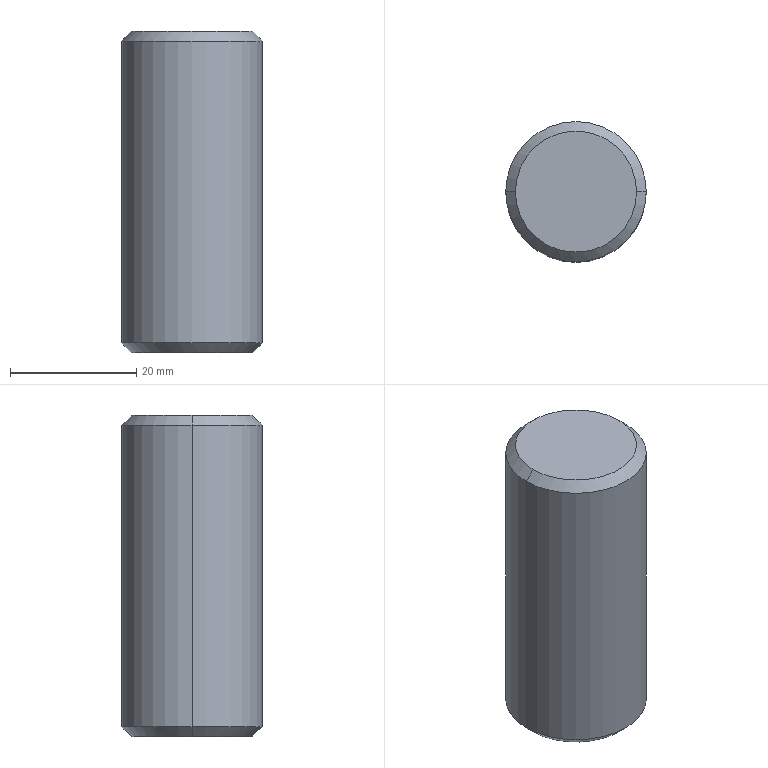Part | SolidWorks | features Chamfer 1, Extrusion 1 | 1 solid | 8 faces | box 22.225 x 22.225 x 50.8 mm | volume 19553 mm3 | cone 4 | cylinder 2 | plane 2 | commonest cylinder face diameters 22.225 x2
STEP:
#1=CARTESIAN_POINT('',(-9.588,0.,-25.4));
#2=VERTEX_POINT('',#1);
#3=CARTESIAN_POINT('',(9.588,0.,-25.4));
#4=VERTEX_POINT('',#3);
#5=CARTESIAN_POINT('',(0.,0.,-25.4));
#6=DIRECTION('',(0.,0.,-1.));
#7=DIRECTION('',(1.,0.,0.));
#8=AXIS2_PLACEMENT_3D('',#5,#6,#7);
#9=CIRCLE('',#8,9.588);
#10=EDGE_CURVE('',#2,#4,#9,.T.);
#11=ORIENTED_EDGE('',*,*,#10,.F.);
#12=CARTESIAN_POINT('',(-11.112,0.,-23.876));
#13=VERTEX_POINT('',#12);
#14=CARTESIAN_POINT('',(-11.112,0.,-23.876));
#15=DIRECTION('',(-0.7071,0.,0.7071));
#16=VECTOR('',#15,1000.);
#17=LINE('',#14,#16);
#18=EDGE_CURVE('',#2,#13,#17,.T.);
#19=ORIENTED_EDGE('',*,*,#18,.T.);
#20=CARTESIAN_POINT('',(11.112,0.,-23.876));
#21=VERTEX_POINT('',#20);
#22=CARTESIAN_POINT('',(0.,0.,-23.876));
#23=DIRECTION('',(0.,0.,1.));
#24=DIRECTION('',(1.,0.,0.));
#25=AXIS2_PLACEMENT_3D('',#22,#23,#24);
#26=CIRCLE('',#25,11.112);
#27=EDGE_CURVE('',#21,#13,#26,.T.);
#28=ORIENTED_EDGE('',*,*,#27,.F.);
#29=CARTESIAN_POINT('',(11.112,0.,-23.876));
#30=DIRECTION('',(0.7071,0.,0.7071));
#31=VECTOR('',#30,1000.);
#32=LINE('',#29,#31);
#33=EDGE_CURVE('',#4,#21,#32,.T.);
#34=ORIENTED_EDGE('',*,*,#33,.F.);
#35=EDGE_LOOP('',(#11,#19,#28,#34));
#36=FACE_OUTER_BOUND('',#35,.T.);
#37=CARTESIAN_POINT('',(0.,0.,-23.876));
#38=DIRECTION('',(0.,0.,1.));
#39=DIRECTION('',(1.,0.,0.));
#40=AXIS2_PLACEMENT_3D('',#37,#38,#39);
#41=CONICAL_SURFACE('',#40,11.112,0.7854);
#42=ADVANCED_FACE('',(#36),#41,.T.);
#43=CARTESIAN_POINT('',(9.588,0.,25.4));
#44=VERTEX_POINT('',#43);
#45=CARTESIAN_POINT('',(-9.588,0.,25.4));
#46=VERTEX_POINT('',#45);
#47=CARTESIAN_POINT('',(0.,0.,25.4));
#48=DIRECTION('',(0.,0.,1.));
#49=DIRECTION('',(1.,0.,0.));
#50=AXIS2_PLACEMENT_3D('',#47,#48,#49);
#51=CIRCLE('',#50,9.588);
#52=EDGE_CURVE('',#44,#46,#51,.T.);
#53=ORIENTED_EDGE('',*,*,#52,.F.);
#54=CARTESIAN_POINT('',(11.112,0.,23.876));
#55=VERTEX_POINT('',#54);
#56=CARTESIAN_POINT('',(9.588,0.,25.4));
#57=DIRECTION('',(0.7071,0.,-0.7071));
#58=VECTOR('',#57,1000.);
#59=LINE('',#56,#58);
#60=EDGE_CURVE('',#44,#55,#59,.T.);
#61=ORIENTED_EDGE('',*,*,#60,.T.);
#62=CARTESIAN_POINT('',(-11.112,0.,23.876));
#63=VERTEX_POINT('',#62);
#64=CARTESIAN_POINT('',(0.,0.,23.876));
#65=DIRECTION('',(0.,0.,-1.));
#66=DIRECTION('',(1.,0.,0.));
#67=AXIS2_PLACEMENT_3D('',#64,#65,#66);
#68=CIRCLE('',#67,11.112);
#69=EDGE_CURVE('',#63,#55,#68,.T.);
#70=ORIENTED_EDGE('',*,*,#69,.F.);
#71=CARTESIAN_POINT('',(-9.588,0.,25.4));
#72=DIRECTION('',(-0.7071,0.,-0.7071));
#73=VECTOR('',#72,1000.);
#74=LINE('',#71,#73);
#75=EDGE_CURVE('',#46,#63,#74,.T.);
#76=ORIENTED_EDGE('',*,*,#75,.F.);
#77=EDGE_LOOP('',(#53,#61,#70,#76));
#78=FACE_OUTER_BOUND('',#77,.T.);
#79=CARTESIAN_POINT('',(0.,0.,25.4));
#80=DIRECTION('',(0.,0.,-1.));
#81=DIRECTION('',(-1.,0.,0.));
#82=AXIS2_PLACEMENT_3D('',#79,#80,#81);
#83=CONICAL_SURFACE('',#82,9.588,0.7854);
#84=ADVANCED_FACE('',(#78),#83,.T.);
#85=ORIENTED_EDGE('',*,*,#69,.T.);
#86=CARTESIAN_POINT('',(11.112,0.,25.4));
#87=DIRECTION('',(0.,0.,-1.));
#88=VECTOR('',#87,1000.);
#89=LINE('',#86,#88);
#90=EDGE_CURVE('',#55,#21,#89,.T.);
#91=ORIENTED_EDGE('',*,*,#90,.T.);
#92=ORIENTED_EDGE('',*,*,#27,.T.);
#93=CARTESIAN_POINT('',(-11.112,0.,25.4));
#94=DIRECTION('',(0.,0.,-1.));
#95=VECTOR('',#94,1000.);
#96=LINE('',#93,#95);
#97=EDGE_CURVE('',#63,#13,#96,.T.);
#98=ORIENTED_EDGE('',*,*,#97,.F.);
#99=EDGE_LOOP('',(#85,#91,#92,#98));
#100=FACE_OUTER_BOUND('',#99,.T.);
#101=CARTESIAN_POINT('',(0.,0.,25.4));
#102=DIRECTION('',(0.,0.,-1.));
#103=DIRECTION('',(-1.,0.,0.));
#104=AXIS2_PLACEMENT_3D('',#101,#102,#103);
#105=CYLINDRICAL_SURFACE('',#104,11.112);
#106=ADVANCED_FACE('',(#100),#105,.T.);
#107=ORIENTED_EDGE('',*,*,#90,.F.);
#108=CARTESIAN_POINT('',(0.,0.,23.876));
#109=DIRECTION('',(0.,0.,-1.));
#110=DIRECTION('',(1.,0.,0.));
#111=AXIS2_PLACEMENT_3D('',#108,#109,#110);
#112=CIRCLE('',#111,11.112);
#113=EDGE_CURVE('',#55,#63,#112,.T.);
#114=ORIENTED_EDGE('',*,*,#113,.T.);
#115=ORIENTED_EDGE('',*,*,#97,.T.);
#116=CARTESIAN_POINT('',(0.,0.,-23.876));
#117=DIRECTION('',(0.,0.,1.));
#118=DIRECTION('',(1.,0.,0.));
#119=AXIS2_PLACEMENT_3D('',#116,#117,#118);
#120=CIRCLE('',#119,11.112);
#121=EDGE_CURVE('',#13,#21,#120,.T.);
#122=ORIENTED_EDGE('',*,*,#121,.T.);
#123=EDGE_LOOP('',(#107,#114,#115,#122));
#124=FACE_OUTER_BOUND('',#123,.T.);
#125=CARTESIAN_POINT('',(0.,0.,25.4));
#126=DIRECTION('',(0.,0.,-1.));
#127=DIRECTION('',(-1.,0.,0.));
#128=AXIS2_PLACEMENT_3D('',#125,#126,#127);
#129=CYLINDRICAL_SURFACE('',#128,11.112);
#130=ADVANCED_FACE('',(#124),#129,.T.);
#131=CARTESIAN_POINT('',(0.,0.,25.4));
#132=DIRECTION('',(0.,0.,1.));
#133=DIRECTION('',(1.,0.,0.));
#134=AXIS2_PLACEMENT_3D('',#131,#132,#133);
#135=CIRCLE('',#134,9.588);
#136=EDGE_CURVE('',#46,#44,#135,.T.);
#137=ORIENTED_EDGE('',*,*,#136,.T.);
#138=ORIENTED_EDGE('',*,*,#52,.T.);
#139=EDGE_LOOP('',(#137,#138));
#140=FACE_OUTER_BOUND('',#139,.T.);
#141=CARTESIAN_POINT('',(0.,0.,25.4));
#142=DIRECTION('',(0.,0.,1.));
#143=DIRECTION('',(1.,0.,0.));
#144=AXIS2_PLACEMENT_3D('',#141,#142,#143);
#145=PLANE('',#144);
#146=ADVANCED_FACE('',(#140),#145,.T.);
#147=CARTESIAN_POINT('',(0.,0.,-25.4));
#148=DIRECTION('',(0.,0.,-1.));
#149=DIRECTION('',(1.,0.,0.));
#150=AXIS2_PLACEMENT_3D('',#147,#148,#149);
#151=CIRCLE('',#150,9.588);
#152=EDGE_CURVE('',#4,#2,#151,.T.);
#153=ORIENTED_EDGE('',*,*,#152,.T.);
#154=ORIENTED_EDGE('',*,*,#10,.T.);
#155=EDGE_LOOP('',(#153,#154));
#156=FACE_OUTER_BOUND('',#155,.T.);
#157=CARTESIAN_POINT('',(0.,0.,-25.4));
#158=DIRECTION('',(0.,0.,1.));
#159=DIRECTION('',(1.,0.,0.));
#160=AXIS2_PLACEMENT_3D('',#157,#158,#159);
#161=PLANE('',#160);
#162=ADVANCED_FACE('',(#156),#161,.F.);
#163=ORIENTED_EDGE('',*,*,#60,.F.);
#164=ORIENTED_EDGE('',*,*,#136,.F.);
#165=ORIENTED_EDGE('',*,*,#75,.T.);
#166=ORIENTED_EDGE('',*,*,#113,.F.);
#167=EDGE_LOOP('',(#163,#164,#165,#166));
#168=FACE_OUTER_BOUND('',#167,.T.);
#169=CARTESIAN_POINT('',(0.,0.,25.4));
#170=DIRECTION('',(0.,0.,-1.));
#171=DIRECTION('',(-1.,0.,0.));
#172=AXIS2_PLACEMENT_3D('',#169,#170,#171);
#173=CONICAL_SURFACE('',#172,9.588,0.7854);
#174=ADVANCED_FACE('',(#168),#173,.T.);
#175=ORIENTED_EDGE('',*,*,#18,.F.);
#176=ORIENTED_EDGE('',*,*,#152,.F.);
#177=ORIENTED_EDGE('',*,*,#33,.T.);
#178=ORIENTED_EDGE('',*,*,#121,.F.);
#179=EDGE_LOOP('',(#175,#176,#177,#178));
#180=FACE_OUTER_BOUND('',#179,.T.);
#181=CARTESIAN_POINT('',(0.,0.,-23.876));
#182=DIRECTION('',(0.,0.,1.));
#183=DIRECTION('',(1.,0.,0.));
#184=AXIS2_PLACEMENT_3D('',#181,#182,#183);
#185=CONICAL_SURFACE('',#184,11.112,0.7854);
#186=ADVANCED_FACE('',(#180),#185,.T.);
#187=CLOSED_SHELL('',(#42,#84,#106,#130,#146,#162,#174,#186));
#188=MANIFOLD_SOLID_BREP('',#187);
#189=CARTESIAN_POINT('',(0.,0.,0.));
#190=DIRECTION('',(0.,0.,1.));
#191=DIRECTION('',(1.,0.,0.));
#192=AXIS2_PLACEMENT_3D('',#189,#190,#191);
#193=(LENGTH_UNIT()NAMED_UNIT(*)SI_UNIT(.MILLI.,.METRE.));
#194=UNCERTAINTY_MEASURE_WITH_UNIT(LENGTH_MEASURE(0.00001),#193,'','');
#195=(NAMED_UNIT(*)PLANE_ANGLE_UNIT()SI_UNIT($,.RADIAN.));
#196=(NAMED_UNIT(*)SI_UNIT($,.STERADIAN.)SOLID_ANGLE_UNIT());
#197=(GEOMETRIC_REPRESENTATION_CONTEXT(3)GLOBAL_UNCERTAINTY_ASSIGNED_CONTEXT((#194))GLOBAL_UNIT_ASSIGNED_CONTEXT((#193,#195,#196))REPRESENTATION_CONTEXT('',''));
#198=ADVANCED_BREP_SHAPE_REPRESENTATION('',(#188,#192),#197);